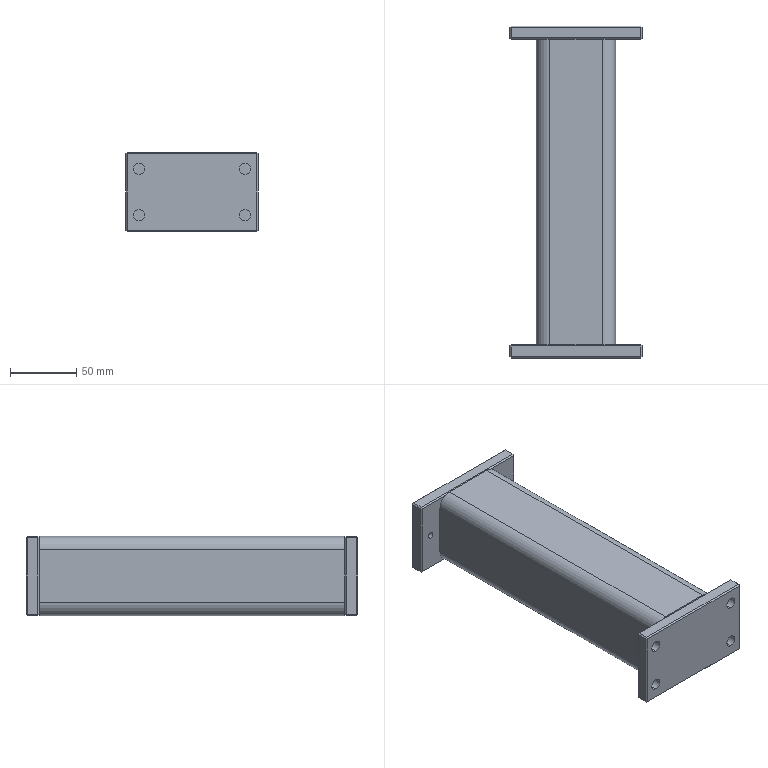Part | SolidWorks | features Chamfer 2, HoleWzd 2, ICE 2, 3DProfileFeature 1, WeldMemberFeat 1, WeldmentFeature 1 | 3 solids | 82 faces | box 100 x 250.5 x 60 mm | volume 355325 mm3 | plane 62 | cylinder 20 | commonest cylinder face diameters 8.6 x8 5 x4 10 x4 20 x4